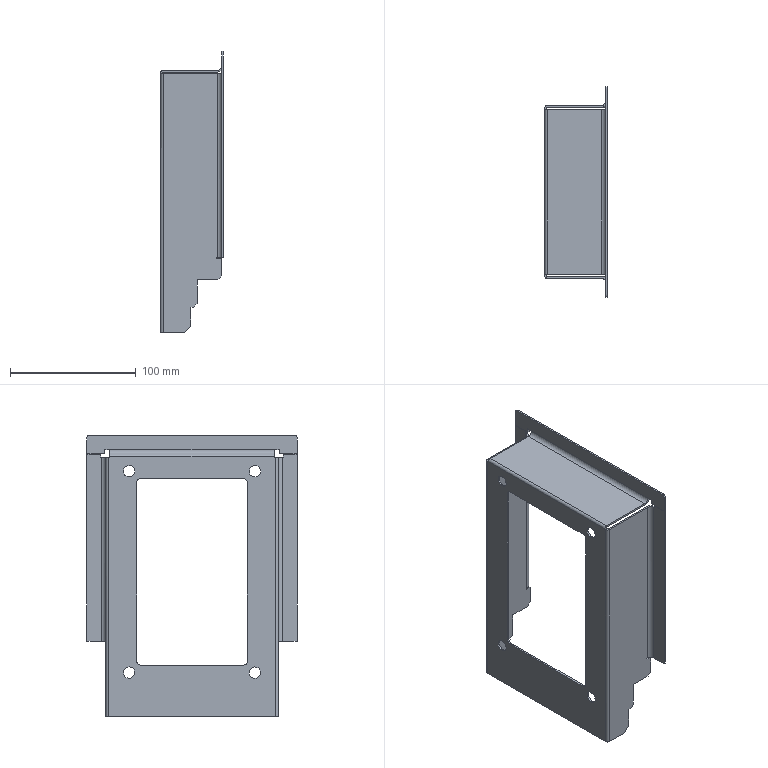Part | STEP file | SYL_0392D6J1SYL0380DJ100-784216 | 1 solid | 110 faces | box 49.95 x 167 x 223.5 mm | volume 65855 mm3 | plane 84 | spline 14 | cylinder 12 | commonest cylinder face diameters 1.1 x3 4 x3 7 x3 9.9 x3